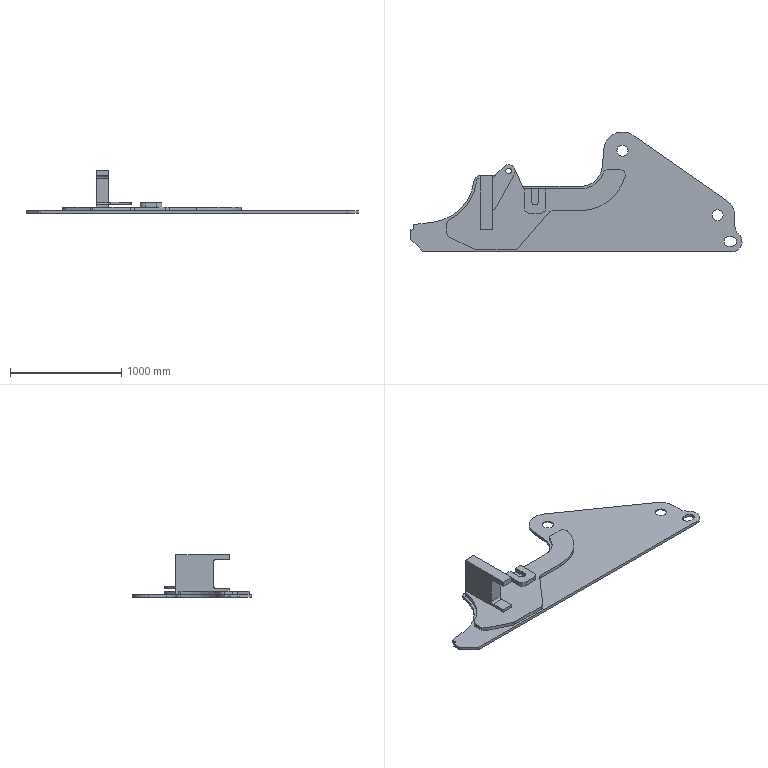Part | NX | features 底座(默认<按焊接>) 2 | 1 solid | 96 faces | box 2987 x 1080 x 386 mm | volume 80381862 mm3 | plane 53 | cylinder 43 | commonest cylinder face diameters 100 x14 20 x4 40 x4 52.37 x2 56.36 x2 87.28 x2